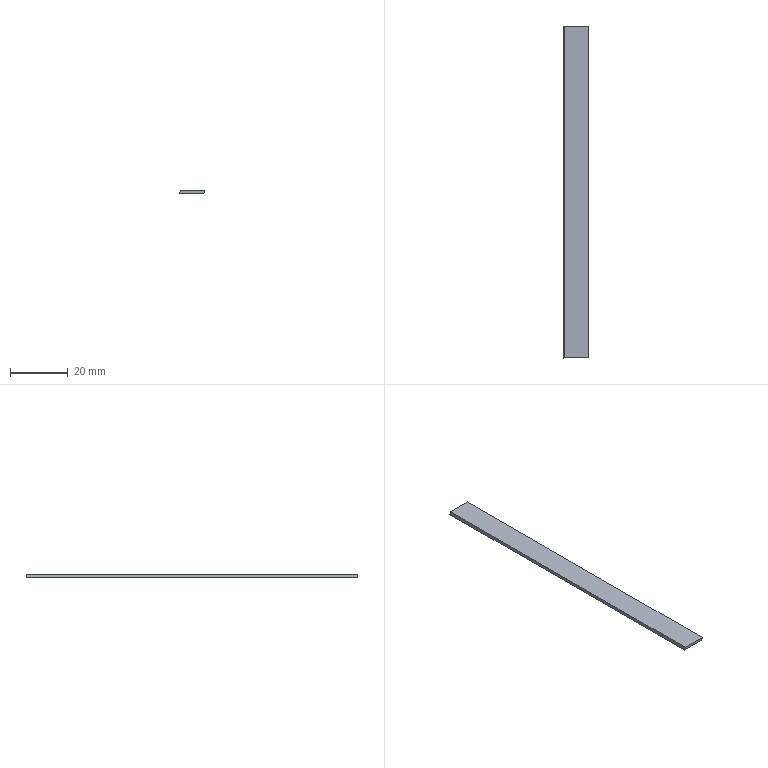Part | SolidWorks | features BaseBody 1 | 1 solid | 6 faces | box 8.595 x 115.104 x 1.056 mm | volume 1022 mm3 | plane 4 | cylinder 2 | commonest cylinder face diameters 97.2 x1 165.792 x1
STEP:
#1=CARTESIAN_POINT('',(-2085.446,1269.344,-1587.891));
#2=VERTEX_POINT('',#1);
#3=CARTESIAN_POINT('',(-2085.687,1269.344,-1588.947));
#4=VERTEX_POINT('',#3);
#5=CARTESIAN_POINT('',(-2132.95,1269.344,-1577.624));
#6=DIRECTION('',(0.,1.,0.));
#7=DIRECTION('',(0.9774,0.,-0.2112));
#8=AXIS2_PLACEMENT_3D('',#5,#6,#7);
#9=CIRCLE('',#8,48.6);
#10=EDGE_CURVE('',#2,#4,#9,.T.);
#11=ORIENTED_EDGE('',*,*,#10,.T.);
#12=CARTESIAN_POINT('',(-2085.687,1154.24,-1588.947));
#13=VERTEX_POINT('',#12);
#14=CARTESIAN_POINT('',(-2085.687,1269.344,-1588.947));
#15=DIRECTION('',(0.,-1.,0.));
#16=VECTOR('',#15,1000.);
#17=LINE('',#14,#16);
#18=EDGE_CURVE('',#4,#13,#17,.T.);
#19=ORIENTED_EDGE('',*,*,#18,.T.);
#20=CARTESIAN_POINT('',(-2085.446,1154.24,-1587.891));
#21=VERTEX_POINT('',#20);
#22=CARTESIAN_POINT('',(-2132.95,1154.24,-1577.624));
#23=DIRECTION('',(0.,-1.,0.));
#24=DIRECTION('',(0.9725,0.,-0.233));
#25=AXIS2_PLACEMENT_3D('',#22,#23,#24);
#26=CIRCLE('',#25,48.6);
#27=EDGE_CURVE('',#13,#21,#26,.T.);
#28=ORIENTED_EDGE('',*,*,#27,.T.);
#29=CARTESIAN_POINT('',(-2085.446,1269.344,-1587.891));
#30=DIRECTION('',(0.,-1.,0.));
#31=VECTOR('',#30,1000.);
#32=LINE('',#29,#31);
#33=EDGE_CURVE('',#2,#21,#32,.T.);
#34=ORIENTED_EDGE('',*,*,#33,.F.);
#35=EDGE_LOOP('',(#11,#19,#28,#34));
#36=FACE_OUTER_BOUND('',#35,.T.);
#37=CARTESIAN_POINT('',(-2132.95,1275.099,-1577.624));
#38=DIRECTION('',(0.,-1.,0.));
#39=DIRECTION('',(0.9485,0.,-0.3168));
#40=AXIS2_PLACEMENT_3D('',#37,#38,#39);
#41=CYLINDRICAL_SURFACE('',#40,48.6);
#42=ADVANCED_FACE('',(#36),#41,.F.);
#43=CARTESIAN_POINT('',(-2077.092,1154.24,-1587.891));
#44=VERTEX_POINT('',#43);
#45=CARTESIAN_POINT('',(-2077.092,1269.344,-1587.891));
#46=VERTEX_POINT('',#45);
#47=CARTESIAN_POINT('',(-2077.092,1154.24,-1587.891));
#48=DIRECTION('',(0.,1.,0.));
#49=VECTOR('',#48,1000.);
#50=LINE('',#47,#49);
#51=EDGE_CURVE('',#44,#46,#50,.T.);
#52=ORIENTED_EDGE('',*,*,#51,.F.);
#53=CARTESIAN_POINT('',(-2077.231,1154.24,-1588.947));
#54=VERTEX_POINT('',#53);
#55=CARTESIAN_POINT('',(-2159.35,1154.24,-1577.624));
#56=DIRECTION('',(0.,-1.,0.));
#57=DIRECTION('',(0.9906,0.,-0.1366));
#58=AXIS2_PLACEMENT_3D('',#55,#56,#57);
#59=CIRCLE('',#58,82.896);
#60=EDGE_CURVE('',#54,#44,#59,.T.);
#61=ORIENTED_EDGE('',*,*,#60,.F.);
#62=CARTESIAN_POINT('',(-2077.231,1269.344,-1588.947));
#63=VERTEX_POINT('',#62);
#64=CARTESIAN_POINT('',(-2077.231,1269.344,-1588.947));
#65=DIRECTION('',(0.,-1.,0.));
#66=VECTOR('',#65,1000.);
#67=LINE('',#64,#66);
#68=EDGE_CURVE('',#63,#54,#67,.T.);
#69=ORIENTED_EDGE('',*,*,#68,.F.);
#70=CARTESIAN_POINT('',(-2159.35,1269.344,-1577.624));
#71=DIRECTION('',(0.,1.,0.));
#72=DIRECTION('',(0.9923,0.,-0.1238));
#73=AXIS2_PLACEMENT_3D('',#70,#71,#72);
#74=CIRCLE('',#73,82.896);
#75=EDGE_CURVE('',#46,#63,#74,.T.);
#76=ORIENTED_EDGE('',*,*,#75,.F.);
#77=EDGE_LOOP('',(#52,#61,#69,#76));
#78=FACE_OUTER_BOUND('',#77,.T.);
#79=CARTESIAN_POINT('',(-2159.35,1275.099,-1577.624));
#80=DIRECTION('',(0.,1.,0.));
#81=DIRECTION('',(0.9993,0.,-0.03689));
#82=AXIS2_PLACEMENT_3D('',#79,#80,#81);
#83=CYLINDRICAL_SURFACE('',#82,82.896);
#84=ADVANCED_FACE('',(#78),#83,.T.);
#85=ORIENTED_EDGE('',*,*,#27,.F.);
#86=CARTESIAN_POINT('',(-2085.687,1154.24,-1588.947));
#87=DIRECTION('',(1.,0.000000003,0.000000002));
#88=VECTOR('',#87,1000.);
#89=LINE('',#86,#88);
#90=EDGE_CURVE('',#13,#54,#89,.T.);
#91=ORIENTED_EDGE('',*,*,#90,.T.);
#92=ORIENTED_EDGE('',*,*,#60,.T.);
#93=CARTESIAN_POINT('',(-2077.092,1154.24,-1587.891));
#94=DIRECTION('',(-1.,-0.000000003,-0.000000002));
#95=VECTOR('',#94,1000.);
#96=LINE('',#93,#95);
#97=EDGE_CURVE('',#44,#21,#96,.T.);
#98=ORIENTED_EDGE('',*,*,#97,.T.);
#99=EDGE_LOOP('',(#85,#91,#92,#98));
#100=FACE_OUTER_BOUND('',#99,.T.);
#101=CARTESIAN_POINT('',(-2086.117,1154.24,-1589.377));
#102=DIRECTION('',(0.,-1.,0.));
#103=DIRECTION('',(0.,0.,-1.));
#104=AXIS2_PLACEMENT_3D('',#101,#102,#103);
#105=PLANE('',#104);
#106=ADVANCED_FACE('',(#100),#105,.T.);
#107=ORIENTED_EDGE('',*,*,#33,.T.);
#108=ORIENTED_EDGE('',*,*,#97,.F.);
#109=ORIENTED_EDGE('',*,*,#51,.T.);
#110=CARTESIAN_POINT('',(-2077.092,1269.344,-1587.891));
#111=DIRECTION('',(-1.,0.000000002,-0.000000003));
#112=VECTOR('',#111,1000.);
#113=LINE('',#110,#112);
#114=EDGE_CURVE('',#46,#2,#113,.T.);
#115=ORIENTED_EDGE('',*,*,#114,.T.);
#116=EDGE_LOOP('',(#107,#108,#109,#115));
#117=FACE_OUTER_BOUND('',#116,.T.);
#118=CARTESIAN_POINT('',(-2091.202,1148.485,-1587.891));
#119=DIRECTION('',(0.,0.,1.));
#120=DIRECTION('',(1.,0.,0.));
#121=AXIS2_PLACEMENT_3D('',#118,#119,#120);
#122=PLANE('',#121);
#123=ADVANCED_FACE('',(#117),#122,.T.);
#124=ORIENTED_EDGE('',*,*,#90,.F.);
#125=ORIENTED_EDGE('',*,*,#18,.F.);
#126=CARTESIAN_POINT('',(-2077.231,1269.344,-1588.947));
#127=DIRECTION('',(-1.,0.000000002,-0.000000002));
#128=VECTOR('',#127,1000.);
#129=LINE('',#126,#128);
#130=EDGE_CURVE('',#63,#4,#129,.T.);
#131=ORIENTED_EDGE('',*,*,#130,.F.);
#132=ORIENTED_EDGE('',*,*,#68,.T.);
#133=EDGE_LOOP('',(#124,#125,#131,#132));
#134=FACE_OUTER_BOUND('',#133,.T.);
#135=CARTESIAN_POINT('',(-2071.475,1148.485,-1588.947));
#136=DIRECTION('',(0.,0.,-1.));
#137=DIRECTION('',(0.,-1.,0.));
#138=AXIS2_PLACEMENT_3D('',#135,#136,#137);
#139=PLANE('',#138);
#140=ADVANCED_FACE('',(#134),#139,.T.);
#141=ORIENTED_EDGE('',*,*,#10,.F.);
#142=ORIENTED_EDGE('',*,*,#114,.F.);
#143=ORIENTED_EDGE('',*,*,#75,.T.);
#144=ORIENTED_EDGE('',*,*,#130,.T.);
#145=EDGE_LOOP('',(#141,#142,#143,#144));
#146=FACE_OUTER_BOUND('',#145,.T.);
#147=CARTESIAN_POINT('',(-2086.117,1269.344,-1589.377));
#148=DIRECTION('',(0.,1.,0.));
#149=DIRECTION('',(1.,0.,0.));
#150=AXIS2_PLACEMENT_3D('',#147,#148,#149);
#151=PLANE('',#150);
#152=ADVANCED_FACE('',(#146),#151,.T.);
#153=CLOSED_SHELL('',(#42,#84,#106,#123,#140,#152));
#154=MANIFOLD_SOLID_BREP('',#153);
#155=CARTESIAN_POINT('',(0.,0.,0.));
#156=DIRECTION('',(0.,0.,1.));
#157=DIRECTION('',(1.,0.,0.));
#158=AXIS2_PLACEMENT_3D('',#155,#156,#157);
#159=(LENGTH_UNIT()NAMED_UNIT(*)SI_UNIT(.MILLI.,.METRE.));
#160=UNCERTAINTY_MEASURE_WITH_UNIT(LENGTH_MEASURE(0.00001),#159,'','');
#161=(NAMED_UNIT(*)PLANE_ANGLE_UNIT()SI_UNIT($,.RADIAN.));
#162=(NAMED_UNIT(*)SI_UNIT($,.STERADIAN.)SOLID_ANGLE_UNIT());
#163=(GEOMETRIC_REPRESENTATION_CONTEXT(3)GLOBAL_UNCERTAINTY_ASSIGNED_CONTEXT((#160))GLOBAL_UNIT_ASSIGNED_CONTEXT((#159,#161,#162))REPRESENTATION_CONTEXT('',''));
#164=ADVANCED_BREP_SHAPE_REPRESENTATION('',(#154,#158),#163);